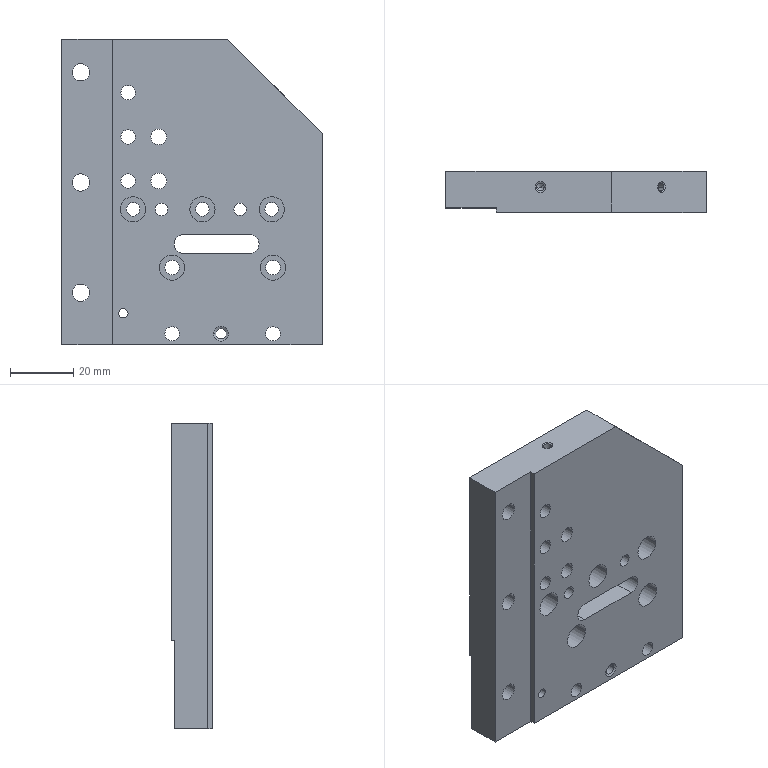Part | NX | 1 solid | 92 faces | box 82.6 x 13 x 97 mm | volume 85503 mm3 | cylinder 61 | plane 21 | cone 10 | commonest cylinder face diameters 4.6 x14 8 x10 4.3 x6 5.5 x6 10 x6 2.5 x4